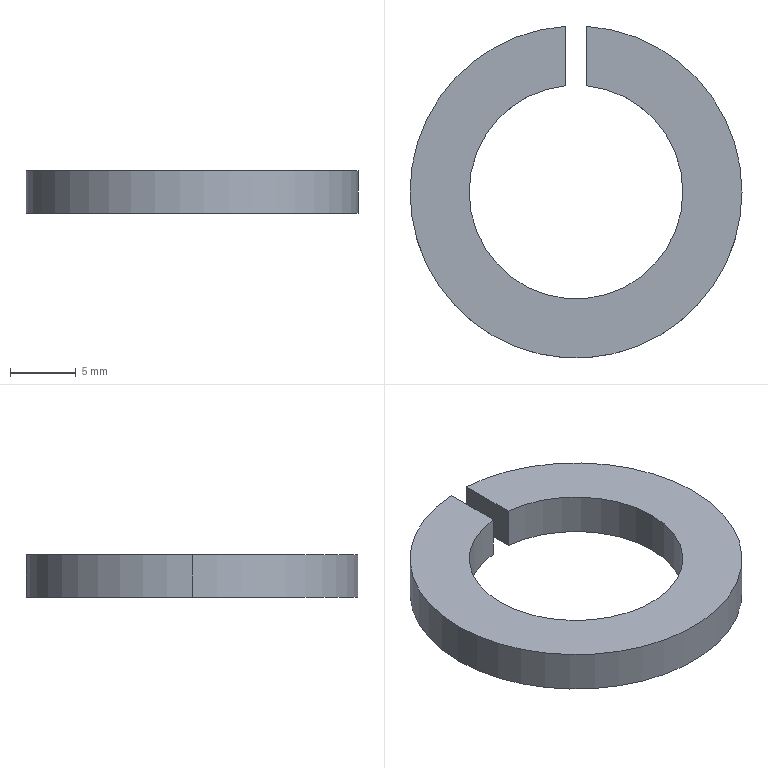Part | SolidWorks | features Extrusion 1 | 1 solid | 10 faces | box 25.172 x 25.146 x 3.2 mm | volume 909.871 mm3 | cylinder 6 | plane 4 | commonest cylinder face diameters 16.2 x3 25.172 x3
STEP:
#1=CARTESIAN_POINT('',(8.1,0.,3.2));
#2=VERTEX_POINT('',#1);
#3=CARTESIAN_POINT('',(-8.1,0.,3.2));
#4=VERTEX_POINT('',#3);
#5=CARTESIAN_POINT('',(0.,0.,3.2));
#6=DIRECTION('',(0.,0.,-1.));
#7=DIRECTION('',(1.,0.,0.));
#8=AXIS2_PLACEMENT_3D('',#5,#6,#7);
#9=CIRCLE('',#8,8.1);
#10=EDGE_CURVE('',#2,#4,#9,.T.);
#11=ORIENTED_EDGE('',*,*,#10,.F.);
#12=CARTESIAN_POINT('',(8.1,0.,0.));
#13=VERTEX_POINT('',#12);
#14=CARTESIAN_POINT('',(8.1,0.,3.2));
#15=DIRECTION('',(0.,0.,-1.));
#16=VECTOR('',#15,1000.);
#17=LINE('',#14,#16);
#18=EDGE_CURVE('',#2,#13,#17,.T.);
#19=ORIENTED_EDGE('',*,*,#18,.T.);
#20=CARTESIAN_POINT('',(-8.1,0.,0.));
#21=VERTEX_POINT('',#20);
#22=CARTESIAN_POINT('',(0.,0.,0.));
#23=DIRECTION('',(0.,0.,-1.));
#24=DIRECTION('',(1.,0.,0.));
#25=AXIS2_PLACEMENT_3D('',#22,#23,#24);
#26=CIRCLE('',#25,8.1);
#27=EDGE_CURVE('',#13,#21,#26,.T.);
#28=ORIENTED_EDGE('',*,*,#27,.T.);
#29=CARTESIAN_POINT('',(-8.1,0.,3.2));
#30=DIRECTION('',(0.,0.,-1.));
#31=VECTOR('',#30,1000.);
#32=LINE('',#29,#31);
#33=EDGE_CURVE('',#4,#21,#32,.T.);
#34=ORIENTED_EDGE('',*,*,#33,.F.);
#35=EDGE_LOOP('',(#11,#19,#28,#34));
#36=FACE_OUTER_BOUND('',#35,.T.);
#37=CARTESIAN_POINT('',(0.,0.,3.2));
#38=DIRECTION('',(0.,0.,-1.));
#39=DIRECTION('',(-1.,0.,0.));
#40=AXIS2_PLACEMENT_3D('',#37,#38,#39);
#41=CYLINDRICAL_SURFACE('',#40,8.1);
#42=ADVANCED_FACE('',(#36),#41,.F.);
#43=CARTESIAN_POINT('',(-0.8,8.06,3.2));
#44=VERTEX_POINT('',#43);
#45=CARTESIAN_POINT('',(0.,0.,3.2));
#46=DIRECTION('',(0.,0.,-1.));
#47=DIRECTION('',(1.,0.,0.));
#48=AXIS2_PLACEMENT_3D('',#45,#46,#47);
#49=CIRCLE('',#48,8.1);
#50=EDGE_CURVE('',#4,#44,#49,.T.);
#51=ORIENTED_EDGE('',*,*,#50,.F.);
#52=ORIENTED_EDGE('',*,*,#33,.T.);
#53=CARTESIAN_POINT('',(-0.8,8.06,0.));
#54=VERTEX_POINT('',#53);
#55=CARTESIAN_POINT('',(0.,0.,0.));
#56=DIRECTION('',(0.,0.,-1.));
#57=DIRECTION('',(1.,0.,0.));
#58=AXIS2_PLACEMENT_3D('',#55,#56,#57);
#59=CIRCLE('',#58,8.1);
#60=EDGE_CURVE('',#21,#54,#59,.T.);
#61=ORIENTED_EDGE('',*,*,#60,.T.);
#62=CARTESIAN_POINT('',(-0.8,8.06,3.2));
#63=DIRECTION('',(0.,0.,-1.));
#64=VECTOR('',#63,1000.);
#65=LINE('',#62,#64);
#66=EDGE_CURVE('',#44,#54,#65,.T.);
#67=ORIENTED_EDGE('',*,*,#66,.F.);
#68=EDGE_LOOP('',(#51,#52,#61,#67));
#69=FACE_OUTER_BOUND('',#68,.T.);
#70=CARTESIAN_POINT('',(0.,0.,3.2));
#71=DIRECTION('',(0.,0.,-1.));
#72=DIRECTION('',(-1.,0.,0.));
#73=AXIS2_PLACEMENT_3D('',#70,#71,#72);
#74=CYLINDRICAL_SURFACE('',#73,8.1);
#75=ADVANCED_FACE('',(#69),#74,.F.);
#76=CARTESIAN_POINT('',(12.586,0.,3.2));
#77=VERTEX_POINT('',#76);
#78=CARTESIAN_POINT('',(0.8,12.56,3.2));
#79=VERTEX_POINT('',#78);
#80=CARTESIAN_POINT('',(0.,0.,3.2));
#81=DIRECTION('',(0.,0.,1.));
#82=DIRECTION('',(1.,0.,0.));
#83=AXIS2_PLACEMENT_3D('',#80,#81,#82);
#84=CIRCLE('',#83,12.586);
#85=EDGE_CURVE('',#77,#79,#84,.T.);
#86=ORIENTED_EDGE('',*,*,#85,.F.);
#87=CARTESIAN_POINT('',(12.586,0.,0.));
#88=VERTEX_POINT('',#87);
#89=CARTESIAN_POINT('',(12.586,0.,3.2));
#90=DIRECTION('',(0.,0.,-1.));
#91=VECTOR('',#90,1000.);
#92=LINE('',#89,#91);
#93=EDGE_CURVE('',#77,#88,#92,.T.);
#94=ORIENTED_EDGE('',*,*,#93,.T.);
#95=CARTESIAN_POINT('',(0.8,12.56,0.));
#96=VERTEX_POINT('',#95);
#97=CARTESIAN_POINT('',(0.,0.,0.));
#98=DIRECTION('',(0.,0.,1.));
#99=DIRECTION('',(1.,0.,0.));
#100=AXIS2_PLACEMENT_3D('',#97,#98,#99);
#101=CIRCLE('',#100,12.586);
#102=EDGE_CURVE('',#88,#96,#101,.T.);
#103=ORIENTED_EDGE('',*,*,#102,.T.);
#104=CARTESIAN_POINT('',(0.8,12.56,3.2));
#105=DIRECTION('',(0.,0.,-1.));
#106=VECTOR('',#105,1000.);
#107=LINE('',#104,#106);
#108=EDGE_CURVE('',#79,#96,#107,.T.);
#109=ORIENTED_EDGE('',*,*,#108,.F.);
#110=EDGE_LOOP('',(#86,#94,#103,#109));
#111=FACE_OUTER_BOUND('',#110,.T.);
#112=CARTESIAN_POINT('',(0.,0.,3.2));
#113=DIRECTION('',(0.,0.,-1.));
#114=DIRECTION('',(-1.,0.,0.));
#115=AXIS2_PLACEMENT_3D('',#112,#113,#114);
#116=CYLINDRICAL_SURFACE('',#115,12.586);
#117=ADVANCED_FACE('',(#111),#116,.T.);
#118=ORIENTED_EDGE('',*,*,#93,.F.);
#119=CARTESIAN_POINT('',(-12.586,0.,3.2));
#120=VERTEX_POINT('',#119);
#121=CARTESIAN_POINT('',(0.,0.,3.2));
#122=DIRECTION('',(0.,0.,1.));
#123=DIRECTION('',(1.,0.,0.));
#124=AXIS2_PLACEMENT_3D('',#121,#122,#123);
#125=CIRCLE('',#124,12.586);
#126=EDGE_CURVE('',#120,#77,#125,.T.);
#127=ORIENTED_EDGE('',*,*,#126,.F.);
#128=CARTESIAN_POINT('',(-12.586,0.,0.));
#129=VERTEX_POINT('',#128);
#130=CARTESIAN_POINT('',(-12.586,0.,3.2));
#131=DIRECTION('',(0.,0.,-1.));
#132=VECTOR('',#131,1000.);
#133=LINE('',#130,#132);
#134=EDGE_CURVE('',#120,#129,#133,.T.);
#135=ORIENTED_EDGE('',*,*,#134,.T.);
#136=CARTESIAN_POINT('',(0.,0.,0.));
#137=DIRECTION('',(0.,0.,1.));
#138=DIRECTION('',(1.,0.,0.));
#139=AXIS2_PLACEMENT_3D('',#136,#137,#138);
#140=CIRCLE('',#139,12.586);
#141=EDGE_CURVE('',#129,#88,#140,.T.);
#142=ORIENTED_EDGE('',*,*,#141,.T.);
#143=EDGE_LOOP('',(#118,#127,#135,#142));
#144=FACE_OUTER_BOUND('',#143,.T.);
#145=CARTESIAN_POINT('',(0.,0.,3.2));
#146=DIRECTION('',(0.,0.,-1.));
#147=DIRECTION('',(-1.,0.,0.));
#148=AXIS2_PLACEMENT_3D('',#145,#146,#147);
#149=CYLINDRICAL_SURFACE('',#148,12.586);
#150=ADVANCED_FACE('',(#144),#149,.T.);
#151=ORIENTED_EDGE('',*,*,#134,.F.);
#152=CARTESIAN_POINT('',(-0.8,12.56,3.2));
#153=VERTEX_POINT('',#152);
#154=CARTESIAN_POINT('',(0.,0.,3.2));
#155=DIRECTION('',(0.,0.,1.));
#156=DIRECTION('',(1.,0.,0.));
#157=AXIS2_PLACEMENT_3D('',#154,#155,#156);
#158=CIRCLE('',#157,12.586);
#159=EDGE_CURVE('',#153,#120,#158,.T.);
#160=ORIENTED_EDGE('',*,*,#159,.F.);
#161=CARTESIAN_POINT('',(-0.8,12.56,0.));
#162=VERTEX_POINT('',#161);
#163=CARTESIAN_POINT('',(-0.8,12.56,3.2));
#164=DIRECTION('',(0.,0.,-1.));
#165=VECTOR('',#164,1000.);
#166=LINE('',#163,#165);
#167=EDGE_CURVE('',#153,#162,#166,.T.);
#168=ORIENTED_EDGE('',*,*,#167,.T.);
#169=CARTESIAN_POINT('',(0.,0.,0.));
#170=DIRECTION('',(0.,0.,1.));
#171=DIRECTION('',(1.,0.,0.));
#172=AXIS2_PLACEMENT_3D('',#169,#170,#171);
#173=CIRCLE('',#172,12.586);
#174=EDGE_CURVE('',#162,#129,#173,.T.);
#175=ORIENTED_EDGE('',*,*,#174,.T.);
#176=EDGE_LOOP('',(#151,#160,#168,#175));
#177=FACE_OUTER_BOUND('',#176,.T.);
#178=CARTESIAN_POINT('',(0.,0.,3.2));
#179=DIRECTION('',(0.,0.,-1.));
#180=DIRECTION('',(-1.,0.,0.));
#181=AXIS2_PLACEMENT_3D('',#178,#179,#180);
#182=CYLINDRICAL_SURFACE('',#181,12.586);
#183=ADVANCED_FACE('',(#177),#182,.T.);
#184=CARTESIAN_POINT('',(0.8,8.06,0.));
#185=VERTEX_POINT('',#184);
#186=CARTESIAN_POINT('',(0.8,12.56,0.));
#187=DIRECTION('',(0.,-1.,0.));
#188=VECTOR('',#187,1000.);
#189=LINE('',#186,#188);
#190=EDGE_CURVE('',#96,#185,#189,.T.);
#191=ORIENTED_EDGE('',*,*,#190,.T.);
#192=CARTESIAN_POINT('',(0.8,8.06,3.2));
#193=VERTEX_POINT('',#192);
#194=CARTESIAN_POINT('',(0.8,8.06,3.2));
#195=DIRECTION('',(0.,0.,-1.));
#196=VECTOR('',#195,1000.);
#197=LINE('',#194,#196);
#198=EDGE_CURVE('',#193,#185,#197,.T.);
#199=ORIENTED_EDGE('',*,*,#198,.F.);
#200=CARTESIAN_POINT('',(0.8,12.56,3.2));
#201=DIRECTION('',(0.,-1.,0.));
#202=VECTOR('',#201,1000.);
#203=LINE('',#200,#202);
#204=EDGE_CURVE('',#79,#193,#203,.T.);
#205=ORIENTED_EDGE('',*,*,#204,.F.);
#206=ORIENTED_EDGE('',*,*,#108,.T.);
#207=EDGE_LOOP('',(#191,#199,#205,#206));
#208=FACE_OUTER_BOUND('',#207,.T.);
#209=CARTESIAN_POINT('',(0.8,12.56,3.2));
#210=DIRECTION('',(1.,0.,0.));
#211=DIRECTION('',(0.,1.,0.));
#212=AXIS2_PLACEMENT_3D('',#209,#210,#211);
#213=PLANE('',#212);
#214=ADVANCED_FACE('',(#208),#213,.F.);
#215=ORIENTED_EDGE('',*,*,#18,.F.);
#216=CARTESIAN_POINT('',(0.,0.,3.2));
#217=DIRECTION('',(0.,0.,-1.));
#218=DIRECTION('',(1.,0.,0.));
#219=AXIS2_PLACEMENT_3D('',#216,#217,#218);
#220=CIRCLE('',#219,8.1);
#221=EDGE_CURVE('',#193,#2,#220,.T.);
#222=ORIENTED_EDGE('',*,*,#221,.F.);
#223=ORIENTED_EDGE('',*,*,#198,.T.);
#224=CARTESIAN_POINT('',(0.,0.,0.));
#225=DIRECTION('',(0.,0.,-1.));
#226=DIRECTION('',(1.,0.,0.));
#227=AXIS2_PLACEMENT_3D('',#224,#225,#226);
#228=CIRCLE('',#227,8.1);
#229=EDGE_CURVE('',#185,#13,#228,.T.);
#230=ORIENTED_EDGE('',*,*,#229,.T.);
#231=EDGE_LOOP('',(#215,#222,#223,#230));
#232=FACE_OUTER_BOUND('',#231,.T.);
#233=CARTESIAN_POINT('',(0.,0.,3.2));
#234=DIRECTION('',(0.,0.,-1.));
#235=DIRECTION('',(-1.,0.,0.));
#236=AXIS2_PLACEMENT_3D('',#233,#234,#235);
#237=CYLINDRICAL_SURFACE('',#236,8.1);
#238=ADVANCED_FACE('',(#232),#237,.F.);
#239=CARTESIAN_POINT('',(-0.8,12.56,0.));
#240=DIRECTION('',(0.,1.,0.));
#241=VECTOR('',#240,1000.);
#242=LINE('',#239,#241);
#243=EDGE_CURVE('',#54,#162,#242,.T.);
#244=ORIENTED_EDGE('',*,*,#243,.T.);
#245=ORIENTED_EDGE('',*,*,#167,.F.);
#246=CARTESIAN_POINT('',(-0.8,12.56,3.2));
#247=DIRECTION('',(0.,1.,0.));
#248=VECTOR('',#247,1000.);
#249=LINE('',#246,#248);
#250=EDGE_CURVE('',#44,#153,#249,.T.);
#251=ORIENTED_EDGE('',*,*,#250,.F.);
#252=ORIENTED_EDGE('',*,*,#66,.T.);
#253=EDGE_LOOP('',(#244,#245,#251,#252));
#254=FACE_OUTER_BOUND('',#253,.T.);
#255=CARTESIAN_POINT('',(-0.8,12.56,3.2));
#256=DIRECTION('',(-1.,0.,0.));
#257=DIRECTION('',(0.,-1.,0.));
#258=AXIS2_PLACEMENT_3D('',#255,#256,#257);
#259=PLANE('',#258);
#260=ADVANCED_FACE('',(#254),#259,.F.);
#261=ORIENTED_EDGE('',*,*,#159,.T.);
#262=ORIENTED_EDGE('',*,*,#126,.T.);
#263=ORIENTED_EDGE('',*,*,#85,.T.);
#264=ORIENTED_EDGE('',*,*,#204,.T.);
#265=ORIENTED_EDGE('',*,*,#221,.T.);
#266=ORIENTED_EDGE('',*,*,#10,.T.);
#267=ORIENTED_EDGE('',*,*,#50,.T.);
#268=ORIENTED_EDGE('',*,*,#250,.T.);
#269=EDGE_LOOP('',(#261,#262,#263,#264,#265,#266,#267,#268));
#270=FACE_OUTER_BOUND('',#269,.T.);
#271=CARTESIAN_POINT('',(0.,0.,3.2));
#272=DIRECTION('',(0.,0.,1.));
#273=DIRECTION('',(1.,0.,0.));
#274=AXIS2_PLACEMENT_3D('',#271,#272,#273);
#275=PLANE('',#274);
#276=ADVANCED_FACE('',(#270),#275,.T.);
#277=ORIENTED_EDGE('',*,*,#174,.F.);
#278=ORIENTED_EDGE('',*,*,#243,.F.);
#279=ORIENTED_EDGE('',*,*,#60,.F.);
#280=ORIENTED_EDGE('',*,*,#27,.F.);
#281=ORIENTED_EDGE('',*,*,#229,.F.);
#282=ORIENTED_EDGE('',*,*,#190,.F.);
#283=ORIENTED_EDGE('',*,*,#102,.F.);
#284=ORIENTED_EDGE('',*,*,#141,.F.);
#285=EDGE_LOOP('',(#277,#278,#279,#280,#281,#282,#283,#284));
#286=FACE_OUTER_BOUND('',#285,.T.);
#287=CARTESIAN_POINT('',(0.,0.,0.));
#288=DIRECTION('',(0.,0.,1.));
#289=DIRECTION('',(1.,0.,0.));
#290=AXIS2_PLACEMENT_3D('',#287,#288,#289);
#291=PLANE('',#290);
#292=ADVANCED_FACE('',(#286),#291,.F.);
#293=CLOSED_SHELL('',(#42,#75,#117,#150,#183,#214,#238,#260,#276,#292));
#294=MANIFOLD_SOLID_BREP('',#293);
#295=CARTESIAN_POINT('',(0.,0.,0.));
#296=DIRECTION('',(0.,0.,1.));
#297=DIRECTION('',(1.,0.,0.));
#298=AXIS2_PLACEMENT_3D('',#295,#296,#297);
#299=(LENGTH_UNIT()NAMED_UNIT(*)SI_UNIT(.MILLI.,.METRE.));
#300=UNCERTAINTY_MEASURE_WITH_UNIT(LENGTH_MEASURE(0.00001),#299,'','');
#301=(NAMED_UNIT(*)PLANE_ANGLE_UNIT()SI_UNIT($,.RADIAN.));
#302=(NAMED_UNIT(*)SI_UNIT($,.STERADIAN.)SOLID_ANGLE_UNIT());
#303=(GEOMETRIC_REPRESENTATION_CONTEXT(3)GLOBAL_UNCERTAINTY_ASSIGNED_CONTEXT((#300))GLOBAL_UNIT_ASSIGNED_CONTEXT((#299,#301,#302))REPRESENTATION_CONTEXT('',''));
#304=ADVANCED_BREP_SHAPE_REPRESENTATION('',(#294,#298),#303);